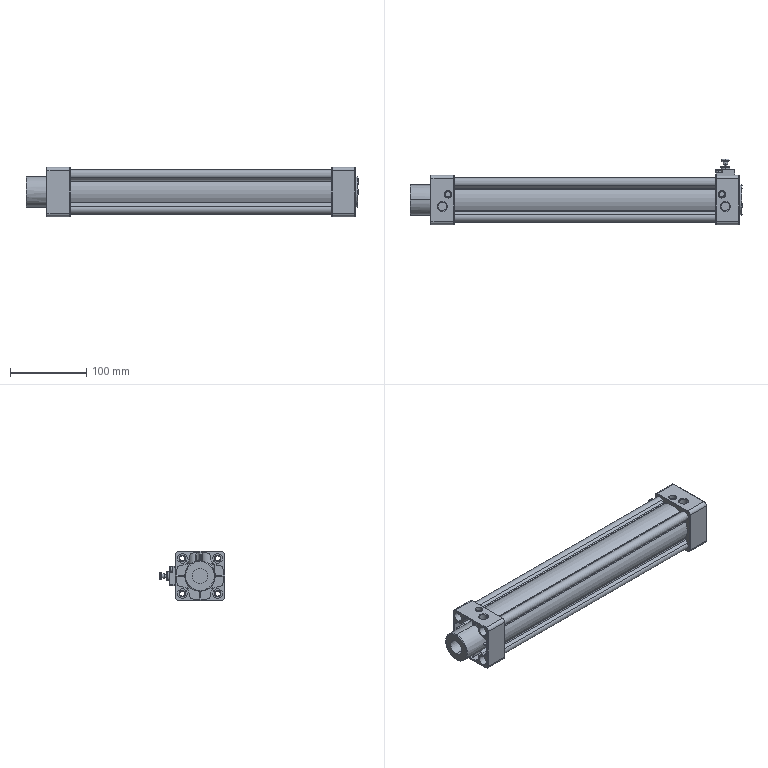Part | SolidWorks | features BaseBody 1 | 1 solid | 345 faces | box 436.5 x 86 x 65 mm | volume 489928 mm3 | cylinder 147 | plane 136 | cone 48 | spline 14 | commonest cylinder face diameters 2 x16 8.7 x16 12 x16 12.7 x16 4 x12 6.8 x8